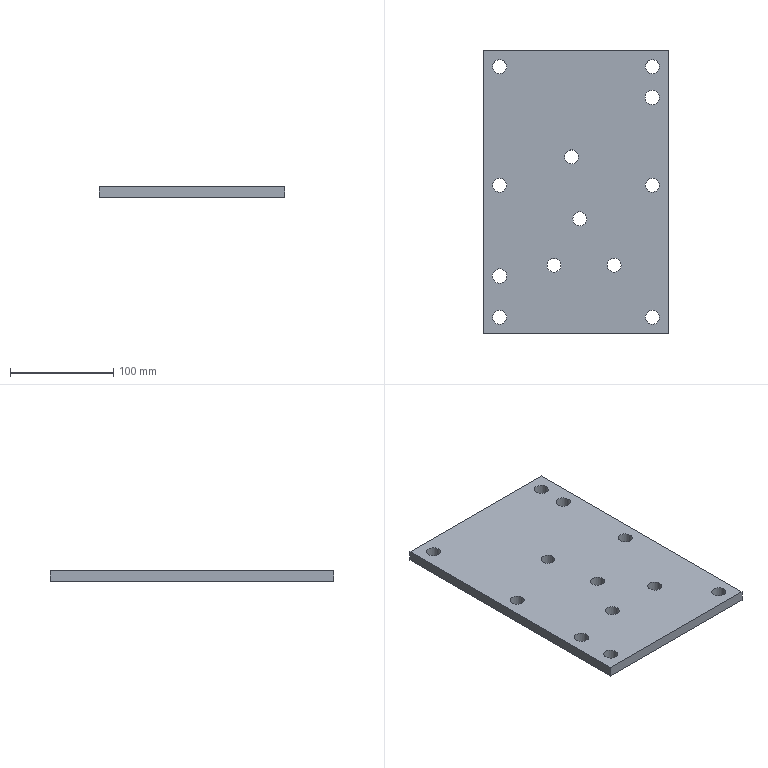Part | STEP file | lll_id2974_x_t | 1 solid | 18 faces | box 180 x 275 x 10 mm | volume 477588 mm3 | cylinder 12 | plane 6 | commonest cylinder face diameters 13.509 x10 14 x2
STEP:
#1=CARTESIAN_POINT('',(1413.393,-159.859,102.5));
#2=VERTEX_POINT('',#1);
#3=CARTESIAN_POINT('',(1420.393,-159.859,102.5));
#4=DIRECTION('',(0.,0.,1.));
#5=DIRECTION('',(-1.,0.,0.));
#6=AXIS2_PLACEMENT_3D('',#3,#4,#5);
#7=CIRCLE('',#6,7.);
#8=EDGE_CURVE('',#2,#2,#7,.T.);
#9=ORIENTED_EDGE('',*,*,#8,.T.);
#10=EDGE_LOOP('',(#9));
#11=FACE_BOUND('',#10,.T.);
#12=CARTESIAN_POINT('',(1413.393,-159.859,92.5));
#13=VERTEX_POINT('',#12);
#14=CARTESIAN_POINT('',(1420.393,-159.859,92.5));
#15=DIRECTION('',(0.,0.,1.));
#16=DIRECTION('',(-1.,0.,0.));
#17=AXIS2_PLACEMENT_3D('',#14,#15,#16);
#18=CIRCLE('',#17,7.);
#19=EDGE_CURVE('',#13,#13,#18,.T.);
#20=ORIENTED_EDGE('',*,*,#19,.F.);
#21=EDGE_LOOP('',(#20));
#22=FACE_BOUND('',#21,.T.);
#23=CARTESIAN_POINT('',(1420.393,-159.859,92.5));
#24=DIRECTION('',(0.,0.,1.));
#25=DIRECTION('',(-1.,0.,0.));
#26=AXIS2_PLACEMENT_3D('',#23,#24,#25);
#27=CYLINDRICAL_SURFACE('',#26,7.);
#28=ADVANCED_FACE('',(#11,#22),#27,.F.);
#29=CARTESIAN_POINT('',(1265.639,-129.859,102.5));
#30=VERTEX_POINT('',#29);
#31=CARTESIAN_POINT('',(1272.393,-129.859,102.5));
#32=DIRECTION('',(0.,0.,-1.));
#33=DIRECTION('',(-1.,0.,0.));
#34=AXIS2_PLACEMENT_3D('',#31,#32,#33);
#35=CIRCLE('',#34,6.755);
#36=EDGE_CURVE('',#30,#30,#35,.T.);
#37=ORIENTED_EDGE('',*,*,#36,.F.);
#38=EDGE_LOOP('',(#37));
#39=FACE_BOUND('',#38,.T.);
#40=CARTESIAN_POINT('',(1265.639,-129.859,92.5));
#41=VERTEX_POINT('',#40);
#42=CARTESIAN_POINT('',(1272.393,-129.859,92.5));
#43=DIRECTION('',(0.,0.,1.));
#44=DIRECTION('',(-1.,0.,0.));
#45=AXIS2_PLACEMENT_3D('',#42,#43,#44);
#46=CIRCLE('',#45,6.755);
#47=EDGE_CURVE('',#41,#41,#46,.T.);
#48=ORIENTED_EDGE('',*,*,#47,.F.);
#49=EDGE_LOOP('',(#48));
#50=FACE_BOUND('',#49,.T.);
#51=CARTESIAN_POINT('',(1272.393,-129.859,92.5));
#52=DIRECTION('',(0.,0.,1.));
#53=DIRECTION('',(-1.,0.,0.));
#54=AXIS2_PLACEMENT_3D('',#51,#52,#53);
#55=CYLINDRICAL_SURFACE('',#54,6.755);
#56=ADVANCED_FACE('',(#39,#50),#55,.F.);
#57=CARTESIAN_POINT('',(1413.639,-129.859,102.5));
#58=VERTEX_POINT('',#57);
#59=CARTESIAN_POINT('',(1420.393,-129.859,102.5));
#60=DIRECTION('',(0.,0.,1.));
#61=DIRECTION('',(-1.,0.,0.));
#62=AXIS2_PLACEMENT_3D('',#59,#60,#61);
#63=CIRCLE('',#62,6.755);
#64=EDGE_CURVE('',#58,#58,#63,.T.);
#65=ORIENTED_EDGE('',*,*,#64,.T.);
#66=EDGE_LOOP('',(#65));
#67=FACE_BOUND('',#66,.T.);
#68=CARTESIAN_POINT('',(1413.639,-129.859,92.5));
#69=VERTEX_POINT('',#68);
#70=CARTESIAN_POINT('',(1420.393,-129.859,92.5));
#71=DIRECTION('',(0.,0.,1.));
#72=DIRECTION('',(-1.,0.,0.));
#73=AXIS2_PLACEMENT_3D('',#70,#71,#72);
#74=CIRCLE('',#73,6.755);
#75=EDGE_CURVE('',#69,#69,#74,.T.);
#76=ORIENTED_EDGE('',*,*,#75,.F.);
#77=EDGE_LOOP('',(#76));
#78=FACE_BOUND('',#77,.T.);
#79=CARTESIAN_POINT('',(1420.393,-129.859,92.5));
#80=DIRECTION('',(0.,0.,1.));
#81=DIRECTION('',(-1.,0.,0.));
#82=AXIS2_PLACEMENT_3D('',#79,#80,#81);
#83=CYLINDRICAL_SURFACE('',#82,6.755);
#84=ADVANCED_FACE('',(#67,#78),#83,.F.);
#85=CARTESIAN_POINT('',(1436.393,-113.859,102.5));
#86=VERTEX_POINT('',#85);
#87=CARTESIAN_POINT('',(1256.393,-113.859,102.5));
#88=VERTEX_POINT('',#87);
#89=CARTESIAN_POINT('',(1346.393,-113.859,102.5));
#90=DIRECTION('',(-1.,0.,0.));
#91=VECTOR('',#90,1.);
#92=LINE('',#89,#91);
#93=EDGE_CURVE('',#86,#88,#92,.T.);
#94=ORIENTED_EDGE('',*,*,#93,.F.);
#95=CARTESIAN_POINT('',(1436.393,-113.859,92.5));
#96=VERTEX_POINT('',#95);
#97=CARTESIAN_POINT('',(1436.393,-113.859,92.5));
#98=DIRECTION('',(0.,0.,1.));
#99=VECTOR('',#98,1.);
#100=LINE('',#97,#99);
#101=EDGE_CURVE('',#96,#86,#100,.T.);
#102=ORIENTED_EDGE('',*,*,#101,.F.);
#103=CARTESIAN_POINT('',(1256.393,-113.859,92.5));
#104=VERTEX_POINT('',#103);
#105=CARTESIAN_POINT('',(1346.393,-113.859,92.5));
#106=DIRECTION('',(-1.,0.,0.));
#107=VECTOR('',#106,1.);
#108=LINE('',#105,#107);
#109=EDGE_CURVE('',#96,#104,#108,.T.);
#110=ORIENTED_EDGE('',*,*,#109,.T.);
#111=CARTESIAN_POINT('',(1256.393,-113.859,92.5));
#112=DIRECTION('',(0.,0.,1.));
#113=VECTOR('',#112,1.);
#114=LINE('',#111,#113);
#115=EDGE_CURVE('',#104,#88,#114,.T.);
#116=ORIENTED_EDGE('',*,*,#115,.T.);
#117=EDGE_LOOP('',(#94,#102,#110,#116));
#118=FACE_OUTER_BOUND('',#117,.T.);
#119=CARTESIAN_POINT('',(1346.393,-113.859,92.5));
#120=DIRECTION('',(0.,1.,0.));
#121=DIRECTION('',(0.,0.,-1.));
#122=AXIS2_PLACEMENT_3D('',#119,#120,#121);
#123=PLANE('',#122);
#124=ADVANCED_FACE('',(#118),#123,.T.);
#125=CARTESIAN_POINT('',(1256.393,-388.859,102.5));
#126=VERTEX_POINT('',#125);
#127=CARTESIAN_POINT('',(1256.393,-251.359,102.5));
#128=DIRECTION('',(0.,1.,0.));
#129=VECTOR('',#128,1.);
#130=LINE('',#127,#129);
#131=EDGE_CURVE('',#126,#88,#130,.T.);
#132=ORIENTED_EDGE('',*,*,#131,.T.);
#133=ORIENTED_EDGE('',*,*,#115,.F.);
#134=CARTESIAN_POINT('',(1256.393,-388.859,92.5));
#135=VERTEX_POINT('',#134);
#136=CARTESIAN_POINT('',(1256.393,-251.359,92.5));
#137=DIRECTION('',(0.,-1.,0.));
#138=VECTOR('',#137,1.);
#139=LINE('',#136,#138);
#140=EDGE_CURVE('',#104,#135,#139,.T.);
#141=ORIENTED_EDGE('',*,*,#140,.T.);
#142=CARTESIAN_POINT('',(1256.393,-388.859,92.5));
#143=DIRECTION('',(0.,0.,1.));
#144=VECTOR('',#143,1.);
#145=LINE('',#142,#144);
#146=EDGE_CURVE('',#135,#126,#145,.T.);
#147=ORIENTED_EDGE('',*,*,#146,.T.);
#148=EDGE_LOOP('',(#132,#133,#141,#147));
#149=FACE_OUTER_BOUND('',#148,.T.);
#150=CARTESIAN_POINT('',(1256.393,-251.359,92.5));
#151=DIRECTION('',(-1.,0.,0.));
#152=DIRECTION('',(0.,0.,-1.));
#153=AXIS2_PLACEMENT_3D('',#150,#151,#152);
#154=PLANE('',#153);
#155=ADVANCED_FACE('',(#149),#154,.T.);
#156=CARTESIAN_POINT('',(1436.393,-388.859,102.5));
#157=VERTEX_POINT('',#156);
#158=CARTESIAN_POINT('',(1346.393,-388.859,102.5));
#159=DIRECTION('',(1.,0.,0.));
#160=VECTOR('',#159,1.);
#161=LINE('',#158,#160);
#162=EDGE_CURVE('',#126,#157,#161,.T.);
#163=ORIENTED_EDGE('',*,*,#162,.F.);
#164=ORIENTED_EDGE('',*,*,#146,.F.);
#165=CARTESIAN_POINT('',(1436.393,-388.859,92.5));
#166=VERTEX_POINT('',#165);
#167=CARTESIAN_POINT('',(1346.393,-388.859,92.5));
#168=DIRECTION('',(1.,0.,0.));
#169=VECTOR('',#168,1.);
#170=LINE('',#167,#169);
#171=EDGE_CURVE('',#135,#166,#170,.T.);
#172=ORIENTED_EDGE('',*,*,#171,.T.);
#173=CARTESIAN_POINT('',(1436.393,-388.859,92.5));
#174=DIRECTION('',(0.,0.,1.));
#175=VECTOR('',#174,1.);
#176=LINE('',#173,#175);
#177=EDGE_CURVE('',#166,#157,#176,.T.);
#178=ORIENTED_EDGE('',*,*,#177,.T.);
#179=EDGE_LOOP('',(#163,#164,#172,#178));
#180=FACE_OUTER_BOUND('',#179,.T.);
#181=CARTESIAN_POINT('',(1346.393,-388.859,92.5));
#182=DIRECTION('',(0.,-1.,0.));
#183=DIRECTION('',(0.,0.,1.));
#184=AXIS2_PLACEMENT_3D('',#181,#182,#183);
#185=PLANE('',#184);
#186=ADVANCED_FACE('',(#180),#185,.T.);
#187=CARTESIAN_POINT('',(1436.393,-251.359,102.5));
#188=DIRECTION('',(0.,1.,0.));
#189=VECTOR('',#188,1.);
#190=LINE('',#187,#189);
#191=EDGE_CURVE('',#157,#86,#190,.T.);
#192=ORIENTED_EDGE('',*,*,#191,.F.);
#193=ORIENTED_EDGE('',*,*,#177,.F.);
#194=CARTESIAN_POINT('',(1436.393,-251.359,92.5));
#195=DIRECTION('',(0.,1.,0.));
#196=VECTOR('',#195,1.);
#197=LINE('',#194,#196);
#198=EDGE_CURVE('',#166,#96,#197,.T.);
#199=ORIENTED_EDGE('',*,*,#198,.T.);
#200=ORIENTED_EDGE('',*,*,#101,.T.);
#201=EDGE_LOOP('',(#192,#193,#199,#200));
#202=FACE_OUTER_BOUND('',#201,.T.);
#203=CARTESIAN_POINT('',(1436.393,-251.359,92.5));
#204=DIRECTION('',(1.,0.,0.));
#205=DIRECTION('',(0.,0.,1.));
#206=AXIS2_PLACEMENT_3D('',#203,#204,#205);
#207=PLANE('',#206);
#208=ADVANCED_FACE('',(#202),#207,.T.);
#209=CARTESIAN_POINT('',(1265.639,-372.859,102.5));
#210=VERTEX_POINT('',#209);
#211=CARTESIAN_POINT('',(1272.393,-372.859,102.5));
#212=DIRECTION('',(0.,0.,1.));
#213=DIRECTION('',(-1.,0.,0.));
#214=AXIS2_PLACEMENT_3D('',#211,#212,#213);
#215=CIRCLE('',#214,6.755);
#216=EDGE_CURVE('',#210,#210,#215,.T.);
#217=ORIENTED_EDGE('',*,*,#216,.T.);
#218=EDGE_LOOP('',(#217));
#219=FACE_BOUND('',#218,.T.);
#220=CARTESIAN_POINT('',(1265.639,-372.859,92.5));
#221=VERTEX_POINT('',#220);
#222=CARTESIAN_POINT('',(1272.393,-372.859,92.5));
#223=DIRECTION('',(0.,0.,1.));
#224=DIRECTION('',(-1.,0.,0.));
#225=AXIS2_PLACEMENT_3D('',#222,#223,#224);
#226=CIRCLE('',#225,6.755);
#227=EDGE_CURVE('',#221,#221,#226,.T.);
#228=ORIENTED_EDGE('',*,*,#227,.F.);
#229=EDGE_LOOP('',(#228));
#230=FACE_BOUND('',#229,.T.);
#231=CARTESIAN_POINT('',(1272.393,-372.859,92.5));
#232=DIRECTION('',(0.,0.,1.));
#233=DIRECTION('',(-1.,0.,0.));
#234=AXIS2_PLACEMENT_3D('',#231,#232,#233);
#235=CYLINDRICAL_SURFACE('',#234,6.755);
#236=ADVANCED_FACE('',(#219,#230),#235,.F.);
#237=CARTESIAN_POINT('',(1413.639,-372.859,102.5));
#238=VERTEX_POINT('',#237);
#239=CARTESIAN_POINT('',(1420.393,-372.859,102.5));
#240=DIRECTION('',(0.,0.,1.));
#241=DIRECTION('',(-1.,0.,0.));
#242=AXIS2_PLACEMENT_3D('',#239,#240,#241);
#243=CIRCLE('',#242,6.755);
#244=EDGE_CURVE('',#238,#238,#243,.T.);
#245=ORIENTED_EDGE('',*,*,#244,.T.);
#246=EDGE_LOOP('',(#245));
#247=FACE_BOUND('',#246,.T.);
#248=CARTESIAN_POINT('',(1413.639,-372.859,92.5));
#249=VERTEX_POINT('',#248);
#250=CARTESIAN_POINT('',(1420.393,-372.859,92.5));
#251=DIRECTION('',(0.,0.,1.));
#252=DIRECTION('',(-1.,0.,0.));
#253=AXIS2_PLACEMENT_3D('',#250,#251,#252);
#254=CIRCLE('',#253,6.755);
#255=EDGE_CURVE('',#249,#249,#254,.T.);
#256=ORIENTED_EDGE('',*,*,#255,.F.);
#257=EDGE_LOOP('',(#256));
#258=FACE_BOUND('',#257,.T.);
#259=CARTESIAN_POINT('',(1420.393,-372.859,92.5));
#260=DIRECTION('',(0.,0.,1.));
#261=DIRECTION('',(-1.,0.,0.));
#262=AXIS2_PLACEMENT_3D('',#259,#260,#261);
#263=CYLINDRICAL_SURFACE('',#262,6.755);
#264=ADVANCED_FACE('',(#247,#258),#263,.F.);
#265=CARTESIAN_POINT('',(1265.393,-332.859,102.5));
#266=VERTEX_POINT('',#265);
#267=CARTESIAN_POINT('',(1272.393,-332.859,102.5));
#268=DIRECTION('',(0.,0.,-1.));
#269=DIRECTION('',(-1.,0.,0.));
#270=AXIS2_PLACEMENT_3D('',#267,#268,#269);
#271=CIRCLE('',#270,7.);
#272=EDGE_CURVE('',#266,#266,#271,.T.);
#273=ORIENTED_EDGE('',*,*,#272,.F.);
#274=EDGE_LOOP('',(#273));
#275=FACE_BOUND('',#274,.T.);
#276=CARTESIAN_POINT('',(1265.393,-332.859,92.5));
#277=VERTEX_POINT('',#276);
#278=CARTESIAN_POINT('',(1272.393,-332.859,92.5));
#279=DIRECTION('',(0.,0.,1.));
#280=DIRECTION('',(-1.,0.,0.));
#281=AXIS2_PLACEMENT_3D('',#278,#279,#280);
#282=CIRCLE('',#281,7.);
#283=EDGE_CURVE('',#277,#277,#282,.T.);
#284=ORIENTED_EDGE('',*,*,#283,.F.);
#285=EDGE_LOOP('',(#284));
#286=FACE_BOUND('',#285,.T.);
#287=CARTESIAN_POINT('',(1272.393,-332.859,92.5));
#288=DIRECTION('',(0.,0.,1.));
#289=DIRECTION('',(-1.,0.,0.));
#290=AXIS2_PLACEMENT_3D('',#287,#288,#289);
#291=CYLINDRICAL_SURFACE('',#290,7.);
#292=ADVANCED_FACE('',(#275,#286),#291,.F.);
#293=CARTESIAN_POINT('',(1265.639,-244.859,102.5));
#294=VERTEX_POINT('',#293);
#295=CARTESIAN_POINT('',(1272.393,-244.859,102.5));
#296=DIRECTION('',(0.,0.,1.));
#297=DIRECTION('',(-1.,0.,0.));
#298=AXIS2_PLACEMENT_3D('',#295,#296,#297);
#299=CIRCLE('',#298,6.755);
#300=EDGE_CURVE('',#294,#294,#299,.T.);
#301=ORIENTED_EDGE('',*,*,#300,.T.);
#302=EDGE_LOOP('',(#301));
#303=FACE_BOUND('',#302,.T.);
#304=CARTESIAN_POINT('',(1265.639,-244.859,92.5));
#305=VERTEX_POINT('',#304);
#306=CARTESIAN_POINT('',(1272.393,-244.859,92.5));
#307=DIRECTION('',(0.,0.,-1.));
#308=DIRECTION('',(-1.,0.,0.));
#309=AXIS2_PLACEMENT_3D('',#306,#307,#308);
#310=CIRCLE('',#309,6.755);
#311=EDGE_CURVE('',#305,#305,#310,.T.);
#312=ORIENTED_EDGE('',*,*,#311,.T.);
#313=EDGE_LOOP('',(#312));
#314=FACE_BOUND('',#313,.T.);
#315=CARTESIAN_POINT('',(1272.393,-244.859,92.5));
#316=DIRECTION('',(0.,0.,1.));
#317=DIRECTION('',(-1.,0.,0.));
#318=AXIS2_PLACEMENT_3D('',#315,#316,#317);
#319=CYLINDRICAL_SURFACE('',#318,6.755);
#320=ADVANCED_FACE('',(#303,#314),#319,.F.);
#321=CARTESIAN_POINT('',(1376.573,-322.359,92.5));
#322=VERTEX_POINT('',#321);
#323=CARTESIAN_POINT('',(1383.328,-322.359,92.5));
#324=DIRECTION('',(0.,0.,-1.));
#325=DIRECTION('',(-1.,0.,0.));
#326=AXIS2_PLACEMENT_3D('',#323,#324,#325);
#327=CIRCLE('',#326,6.755);
#328=EDGE_CURVE('',#322,#322,#327,.T.);
#329=ORIENTED_EDGE('',*,*,#328,.F.);
#330=EDGE_LOOP('',(#329));
#331=FACE_BOUND('',#330,.T.);
#332=CARTESIAN_POINT('',(1335.307,-217.359,92.5));
#333=VERTEX_POINT('',#332);
#334=CARTESIAN_POINT('',(1342.062,-217.359,92.5));
#335=DIRECTION('',(0.,0.,-1.));
#336=DIRECTION('',(-1.,0.,0.));
#337=AXIS2_PLACEMENT_3D('',#334,#335,#336);
#338=CIRCLE('',#337,6.755);
#339=EDGE_CURVE('',#333,#333,#338,.T.);
#340=ORIENTED_EDGE('',*,*,#339,.F.);
#341=EDGE_LOOP('',(#340));
#342=FACE_BOUND('',#341,.T.);
#343=CARTESIAN_POINT('',(1318.307,-322.359,92.5));
#344=VERTEX_POINT('',#343);
#345=CARTESIAN_POINT('',(1325.062,-322.359,92.5));
#346=DIRECTION('',(0.,0.,-1.));
#347=DIRECTION('',(-1.,0.,0.));
#348=AXIS2_PLACEMENT_3D('',#345,#346,#347);
#349=CIRCLE('',#348,6.755);
#350=EDGE_CURVE('',#344,#344,#349,.T.);
#351=ORIENTED_EDGE('',*,*,#350,.F.);
#352=EDGE_LOOP('',(#351));
#353=FACE_BOUND('',#352,.T.);
#354=CARTESIAN_POINT('',(1343.307,-277.359,92.5));
#355=VERTEX_POINT('',#354);
#356=CARTESIAN_POINT('',(1350.062,-277.359,92.5));
#357=DIRECTION('',(0.,0.,-1.));
#358=DIRECTION('',(-1.,0.,0.));
#359=AXIS2_PLACEMENT_3D('',#356,#357,#358);
#360=CIRCLE('',#359,6.755);
#361=EDGE_CURVE('',#355,#355,#360,.T.);
#362=ORIENTED_EDGE('',*,*,#361,.F.);
#363=EDGE_LOOP('',(#362));
#364=FACE_BOUND('',#363,.T.);
#365=CARTESIAN_POINT('',(1413.639,-244.859,92.5));
#366=VERTEX_POINT('',#365);
#367=CARTESIAN_POINT('',(1420.393,-244.859,92.5));
#368=DIRECTION('',(0.,0.,-1.));
#369=DIRECTION('',(-1.,0.,0.));
#370=AXIS2_PLACEMENT_3D('',#367,#368,#369);
#371=CIRCLE('',#370,6.755);
#372=EDGE_CURVE('',#366,#366,#371,.T.);
#373=ORIENTED_EDGE('',*,*,#372,.F.);
#374=EDGE_LOOP('',(#373));
#375=FACE_BOUND('',#374,.T.);
#376=ORIENTED_EDGE('',*,*,#311,.F.);
#377=EDGE_LOOP('',(#376));
#378=FACE_BOUND('',#377,.T.);
#379=ORIENTED_EDGE('',*,*,#283,.T.);
#380=EDGE_LOOP('',(#379));
#381=FACE_BOUND('',#380,.T.);
#382=ORIENTED_EDGE('',*,*,#255,.T.);
#383=EDGE_LOOP('',(#382));
#384=FACE_BOUND('',#383,.T.);
#385=ORIENTED_EDGE('',*,*,#227,.T.);
#386=EDGE_LOOP('',(#385));
#387=FACE_BOUND('',#386,.T.);
#388=ORIENTED_EDGE('',*,*,#140,.F.);
#389=ORIENTED_EDGE('',*,*,#109,.F.);
#390=ORIENTED_EDGE('',*,*,#198,.F.);
#391=ORIENTED_EDGE('',*,*,#171,.F.);
#392=EDGE_LOOP('',(#388,#389,#390,#391));
#393=FACE_BOUND('',#392,.T.);
#394=ORIENTED_EDGE('',*,*,#75,.T.);
#395=EDGE_LOOP('',(#394));
#396=FACE_BOUND('',#395,.T.);
#397=ORIENTED_EDGE('',*,*,#47,.T.);
#398=EDGE_LOOP('',(#397));
#399=FACE_BOUND('',#398,.T.);
#400=ORIENTED_EDGE('',*,*,#19,.T.);
#401=EDGE_LOOP('',(#400));
#402=FACE_BOUND('',#401,.T.);
#403=CARTESIAN_POINT('',(1346.393,-251.359,92.5));
#404=DIRECTION('',(0.,0.,-1.));
#405=DIRECTION('',(1.,0.,0.));
#406=AXIS2_PLACEMENT_3D('',#403,#404,#405);
#407=PLANE('',#406);
#408=ADVANCED_FACE('',(#331,#342,#353,#364,#375,#378,#381,#384,#387,#393,#396,#399,#402),#407,.T.);
#409=CARTESIAN_POINT('',(1413.639,-244.859,102.5));
#410=VERTEX_POINT('',#409);
#411=CARTESIAN_POINT('',(1420.393,-244.859,102.5));
#412=DIRECTION('',(0.,0.,1.));
#413=DIRECTION('',(-1.,0.,0.));
#414=AXIS2_PLACEMENT_3D('',#411,#412,#413);
#415=CIRCLE('',#414,6.755);
#416=EDGE_CURVE('',#410,#410,#415,.T.);
#417=ORIENTED_EDGE('',*,*,#416,.T.);
#418=EDGE_LOOP('',(#417));
#419=FACE_BOUND('',#418,.T.);
#420=ORIENTED_EDGE('',*,*,#372,.T.);
#421=EDGE_LOOP('',(#420));
#422=FACE_BOUND('',#421,.T.);
#423=CARTESIAN_POINT('',(1420.393,-244.859,92.5));
#424=DIRECTION('',(0.,0.,1.));
#425=DIRECTION('',(-1.,0.,0.));
#426=AXIS2_PLACEMENT_3D('',#423,#424,#425);
#427=CYLINDRICAL_SURFACE('',#426,6.755);
#428=ADVANCED_FACE('',(#419,#422),#427,.F.);
#429=CARTESIAN_POINT('',(1376.573,-322.359,102.5));
#430=VERTEX_POINT('',#429);
#431=CARTESIAN_POINT('',(1383.328,-322.359,102.5));
#432=DIRECTION('',(0.,0.,-1.));
#433=DIRECTION('',(-1.,0.,0.));
#434=AXIS2_PLACEMENT_3D('',#431,#432,#433);
#435=CIRCLE('',#434,6.755);
#436=EDGE_CURVE('',#430,#430,#435,.T.);
#437=ORIENTED_EDGE('',*,*,#436,.T.);
#438=EDGE_LOOP('',(#437));
#439=FACE_BOUND('',#438,.T.);
#440=CARTESIAN_POINT('',(1335.307,-217.359,102.5));
#441=VERTEX_POINT('',#440);
#442=CARTESIAN_POINT('',(1342.062,-217.359,102.5));
#443=DIRECTION('',(0.,0.,-1.));
#444=DIRECTION('',(-1.,0.,0.));
#445=AXIS2_PLACEMENT_3D('',#442,#443,#444);
#446=CIRCLE('',#445,6.755);
#447=EDGE_CURVE('',#441,#441,#446,.T.);
#448=ORIENTED_EDGE('',*,*,#447,.T.);
#449=EDGE_LOOP('',(#448));
#450=FACE_BOUND('',#449,.T.);
#451=CARTESIAN_POINT('',(1318.307,-322.359,102.5));
#452=VERTEX_POINT('',#451);
#453=CARTESIAN_POINT('',(1325.062,-322.359,102.5));
#454=DIRECTION('',(0.,0.,-1.));
#455=DIRECTION('',(-1.,0.,0.));
#456=AXIS2_PLACEMENT_3D('',#453,#454,#455);
#457=CIRCLE('',#456,6.755);
#458=EDGE_CURVE('',#452,#452,#457,.T.);
#459=ORIENTED_EDGE('',*,*,#458,.T.);
#460=EDGE_LOOP('',(#459));
#461=FACE_BOUND('',#460,.T.);
#462=CARTESIAN_POINT('',(1343.307,-277.359,102.5));
#463=VERTEX_POINT('',#462);
#464=CARTESIAN_POINT('',(1350.062,-277.359,102.5));
#465=DIRECTION('',(0.,0.,-1.));
#466=DIRECTION('',(-1.,0.,0.));
#467=AXIS2_PLACEMENT_3D('',#464,#465,#466);
#468=CIRCLE('',#467,6.755);
#469=EDGE_CURVE('',#463,#463,#468,.T.);
#470=ORIENTED_EDGE('',*,*,#469,.T.);
#471=EDGE_LOOP('',(#470));
#472=FACE_BOUND('',#471,.T.);
#473=ORIENTED_EDGE('',*,*,#36,.T.);
#474=EDGE_LOOP('',(#473));
#475=FACE_BOUND('',#474,.T.);
#476=ORIENTED_EDGE('',*,*,#216,.F.);
#477=EDGE_LOOP('',(#476));
#478=FACE_BOUND('',#477,.T.);
#479=ORIENTED_EDGE('',*,*,#272,.T.);
#480=EDGE_LOOP('',(#479));
#481=FACE_BOUND('',#480,.T.);
#482=ORIENTED_EDGE('',*,*,#416,.F.);
#483=EDGE_LOOP('',(#482));
#484=FACE_BOUND('',#483,.T.);
#485=ORIENTED_EDGE('',*,*,#300,.F.);
#486=EDGE_LOOP('',(#485));
#487=FACE_BOUND('',#486,.T.);
#488=ORIENTED_EDGE('',*,*,#244,.F.);
#489=EDGE_LOOP('',(#488));
#490=FACE_BOUND('',#489,.T.);
#491=ORIENTED_EDGE('',*,*,#191,.T.);
#492=ORIENTED_EDGE('',*,*,#93,.T.);
#493=ORIENTED_EDGE('',*,*,#131,.F.);
#494=ORIENTED_EDGE('',*,*,#162,.T.);
#495=EDGE_LOOP('',(#491,#492,#493,#494));
#496=FACE_BOUND('',#495,.T.);
#497=ORIENTED_EDGE('',*,*,#64,.F.);
#498=EDGE_LOOP('',(#497));
#499=FACE_BOUND('',#498,.T.);
#500=ORIENTED_EDGE('',*,*,#8,.F.);
#501=EDGE_LOOP('',(#500));
#502=FACE_BOUND('',#501,.T.);
#503=CARTESIAN_POINT('',(1353.5,0.,102.5));
#504=DIRECTION('',(0.,0.,-1.));
#505=DIRECTION('',(-1.,0.,0.));
#506=AXIS2_PLACEMENT_3D('',#503,#504,#505);
#507=PLANE('',#506);
#508=ADVANCED_FACE('',(#439,#450,#461,#472,#475,#478,#481,#484,#487,#490,#496,#499,#502),#507,.F.);
#509=ORIENTED_EDGE('',*,*,#361,.T.);
#510=EDGE_LOOP('',(#509));
#511=FACE_BOUND('',#510,.T.);
#512=ORIENTED_EDGE('',*,*,#469,.F.);
#513=EDGE_LOOP('',(#512));
#514=FACE_BOUND('',#513,.T.);
#515=CARTESIAN_POINT('',(1350.062,-277.359,337.5));
#516=DIRECTION('',(0.,0.,-1.));
#517=DIRECTION('',(-1.,0.,0.));
#518=AXIS2_PLACEMENT_3D('',#515,#516,#517);
#519=CYLINDRICAL_SURFACE('',#518,6.755);
#520=ADVANCED_FACE('',(#511,#514),#519,.F.);
#521=ORIENTED_EDGE('',*,*,#350,.T.);
#522=EDGE_LOOP('',(#521));
#523=FACE_BOUND('',#522,.T.);
#524=ORIENTED_EDGE('',*,*,#458,.F.);
#525=EDGE_LOOP('',(#524));
#526=FACE_BOUND('',#525,.T.);
#527=CARTESIAN_POINT('',(1325.062,-322.359,337.5));
#528=DIRECTION('',(0.,0.,-1.));
#529=DIRECTION('',(-1.,0.,0.));
#530=AXIS2_PLACEMENT_3D('',#527,#528,#529);
#531=CYLINDRICAL_SURFACE('',#530,6.755);
#532=ADVANCED_FACE('',(#523,#526),#531,.F.);
#533=ORIENTED_EDGE('',*,*,#339,.T.);
#534=EDGE_LOOP('',(#533));
#535=FACE_BOUND('',#534,.T.);
#536=ORIENTED_EDGE('',*,*,#447,.F.);
#537=EDGE_LOOP('',(#536));
#538=FACE_BOUND('',#537,.T.);
#539=CARTESIAN_POINT('',(1342.062,-217.359,337.5));
#540=DIRECTION('',(0.,0.,-1.));
#541=DIRECTION('',(-1.,0.,0.));
#542=AXIS2_PLACEMENT_3D('',#539,#540,#541);
#543=CYLINDRICAL_SURFACE('',#542,6.755);
#544=ADVANCED_FACE('',(#535,#538),#543,.F.);
#545=ORIENTED_EDGE('',*,*,#328,.T.);
#546=EDGE_LOOP('',(#545));
#547=FACE_BOUND('',#546,.T.);
#548=ORIENTED_EDGE('',*,*,#436,.F.);
#549=EDGE_LOOP('',(#548));
#550=FACE_BOUND('',#549,.T.);
#551=CARTESIAN_POINT('',(1383.328,-322.359,337.5));
#552=DIRECTION('',(0.,0.,-1.));
#553=DIRECTION('',(-1.,0.,0.));
#554=AXIS2_PLACEMENT_3D('',#551,#552,#553);
#555=CYLINDRICAL_SURFACE('',#554,6.755);
#556=ADVANCED_FACE('',(#547,#550),#555,.F.);
#557=CLOSED_SHELL('',(#28,#56,#84,#124,#155,#186,#208,#236,#264,#292,#320,#408,#428,#508,#520,#532,#544,#556));
#558=MANIFOLD_SOLID_BREP('',#557);
#559=(LENGTH_UNIT()NAMED_UNIT(*)SI_UNIT(.MILLI.,.METRE.));
#560=UNCERTAINTY_MEASURE_WITH_UNIT(LENGTH_MEASURE(0.00002),#559,'','');
#561=(NAMED_UNIT(*)PLANE_ANGLE_UNIT()SI_UNIT($,.RADIAN.));
#562=PLANE_ANGLE_MEASURE_WITH_UNIT(PLANE_ANGLE_MEASURE(0.01745),#561);
#563=DIMENSIONAL_EXPONENTS(0.,0.,0.,0.,0.,0.,0.);
#564=(CONVERSION_BASED_UNIT('DEGREE',#562)NAMED_UNIT(#563)PLANE_ANGLE_UNIT());
#565=(NAMED_UNIT(*)SI_UNIT($,.STERADIAN.)SOLID_ANGLE_UNIT());
#566=(GEOMETRIC_REPRESENTATION_CONTEXT(3)GLOBAL_UNCERTAINTY_ASSIGNED_CONTEXT((#560))GLOBAL_UNIT_ASSIGNED_CONTEXT((#559,#564,#565))REPRESENTATION_CONTEXT('',''));
#567=ADVANCED_BREP_SHAPE_REPRESENTATION('',(#558),#566);